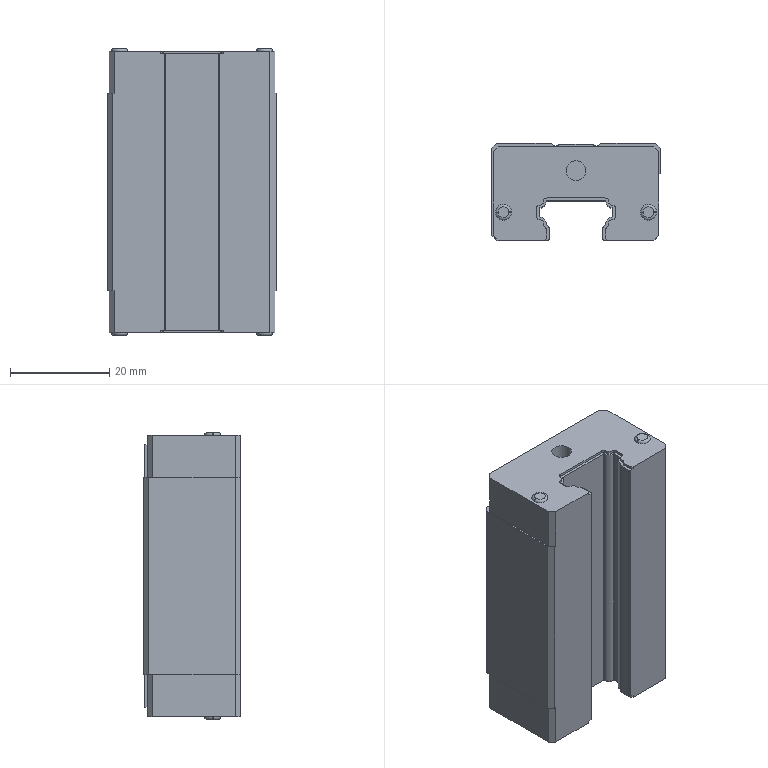Part | NX | 1 solid | 150 faces | box 34 x 19.5 x 57.8 mm | volume 30498 mm3 | plane 82 | cylinder 52 | spline 8 | torus 8 | commonest cylinder face diameters 1.6 x16 0.46 x8 2.1 x8 4 x6 0.6 x4 0.74 x4